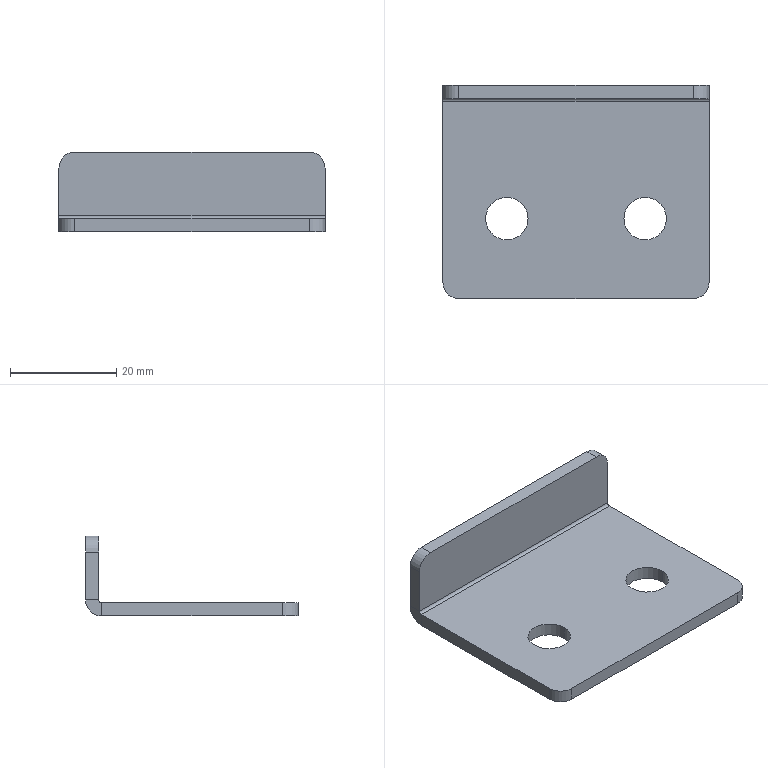Part | SolidWorks | features BaseBody 1 | 1 solid | 22 faces | box 50 x 40 x 15 mm | volume 6198 mm3 | plane 12 | cylinder 10 | commonest cylinder face diameters 6 x5 8 x4 1 x1
STEP:
#1=CARTESIAN_POINT('',(-17.,-5.,-2.5));
#2=VERTEX_POINT('',#1);
#3=CARTESIAN_POINT('',(-17.,-5.,0.));
#4=VERTEX_POINT('',#3);
#5=CARTESIAN_POINT('',(-17.,-5.,-2.5));
#6=DIRECTION('',(0.,0.,1.));
#7=VECTOR('',#6,1000.);
#8=LINE('',#5,#7);
#9=EDGE_CURVE('',#2,#4,#8,.T.);
#10=ORIENTED_EDGE('',*,*,#9,.F.);
#11=CARTESIAN_POINT('',(-9.,-5.,-2.5));
#12=VERTEX_POINT('',#11);
#13=CARTESIAN_POINT('',(-13.,-5.,-2.5));
#14=DIRECTION('',(0.,0.,1.));
#15=DIRECTION('',(1.,0.,0.));
#16=AXIS2_PLACEMENT_3D('',#13,#14,#15);
#17=CIRCLE('',#16,4.);
#18=EDGE_CURVE('',#12,#2,#17,.T.);
#19=ORIENTED_EDGE('',*,*,#18,.F.);
#20=CARTESIAN_POINT('',(-9.,-5.,0.));
#21=VERTEX_POINT('',#20);
#22=CARTESIAN_POINT('',(-9.,-5.,-2.5));
#23=DIRECTION('',(0.,0.,1.));
#24=VECTOR('',#23,1000.);
#25=LINE('',#22,#24);
#26=EDGE_CURVE('',#12,#21,#25,.T.);
#27=ORIENTED_EDGE('',*,*,#26,.T.);
#28=CARTESIAN_POINT('',(-13.,-5.,0.));
#29=DIRECTION('',(0.,0.,1.));
#30=DIRECTION('',(1.,0.,0.));
#31=AXIS2_PLACEMENT_3D('',#28,#29,#30);
#32=CIRCLE('',#31,4.);
#33=EDGE_CURVE('',#21,#4,#32,.T.);
#34=ORIENTED_EDGE('',*,*,#33,.T.);
#35=EDGE_LOOP('',(#10,#19,#27,#34));
#36=FACE_OUTER_BOUND('',#35,.T.);
#37=CARTESIAN_POINT('',(-13.,-5.,-2.5));
#38=DIRECTION('',(0.,0.,1.));
#39=DIRECTION('',(1.,0.,0.));
#40=AXIS2_PLACEMENT_3D('',#37,#38,#39);
#41=CYLINDRICAL_SURFACE('',#40,4.);
#42=ADVANCED_FACE('',(#36),#41,.F.);
#43=CARTESIAN_POINT('',(9.,-5.,-2.5));
#44=VERTEX_POINT('',#43);
#45=CARTESIAN_POINT('',(9.,-5.,0.));
#46=VERTEX_POINT('',#45);
#47=CARTESIAN_POINT('',(9.,-5.,-2.5));
#48=DIRECTION('',(0.,0.,1.));
#49=VECTOR('',#48,1000.);
#50=LINE('',#47,#49);
#51=EDGE_CURVE('',#44,#46,#50,.T.);
#52=ORIENTED_EDGE('',*,*,#51,.F.);
#53=CARTESIAN_POINT('',(17.,-5.,-2.5));
#54=VERTEX_POINT('',#53);
#55=CARTESIAN_POINT('',(13.,-5.,-2.5));
#56=DIRECTION('',(0.,0.,1.));
#57=DIRECTION('',(1.,0.,0.));
#58=AXIS2_PLACEMENT_3D('',#55,#56,#57);
#59=CIRCLE('',#58,4.);
#60=EDGE_CURVE('',#54,#44,#59,.T.);
#61=ORIENTED_EDGE('',*,*,#60,.F.);
#62=CARTESIAN_POINT('',(17.,-5.,0.));
#63=VERTEX_POINT('',#62);
#64=CARTESIAN_POINT('',(17.,-5.,-2.5));
#65=DIRECTION('',(0.,0.,1.));
#66=VECTOR('',#65,1000.);
#67=LINE('',#64,#66);
#68=EDGE_CURVE('',#54,#63,#67,.T.);
#69=ORIENTED_EDGE('',*,*,#68,.T.);
#70=CARTESIAN_POINT('',(13.,-5.,0.));
#71=DIRECTION('',(0.,0.,1.));
#72=DIRECTION('',(1.,0.,0.));
#73=AXIS2_PLACEMENT_3D('',#70,#71,#72);
#74=CIRCLE('',#73,4.);
#75=EDGE_CURVE('',#63,#46,#74,.T.);
#76=ORIENTED_EDGE('',*,*,#75,.T.);
#77=EDGE_LOOP('',(#52,#61,#69,#76));
#78=FACE_OUTER_BOUND('',#77,.T.);
#79=CARTESIAN_POINT('',(13.,-5.,-2.5));
#80=DIRECTION('',(0.,0.,1.));
#81=DIRECTION('',(1.,0.,0.));
#82=AXIS2_PLACEMENT_3D('',#79,#80,#81);
#83=CYLINDRICAL_SURFACE('',#82,4.);
#84=ADVANCED_FACE('',(#78),#83,.F.);
#85=CARTESIAN_POINT('',(-25.,20.,9.5));
#86=VERTEX_POINT('',#85);
#87=CARTESIAN_POINT('',(-22.,20.,12.5));
#88=VERTEX_POINT('',#87);
#89=CARTESIAN_POINT('',(-22.,20.,9.5));
#90=DIRECTION('',(0.,1.,0.));
#91=DIRECTION('',(0.,0.,-1.));
#92=AXIS2_PLACEMENT_3D('',#89,#90,#91);
#93=CIRCLE('',#92,3.);
#94=EDGE_CURVE('',#86,#88,#93,.T.);
#95=ORIENTED_EDGE('',*,*,#94,.F.);
#96=CARTESIAN_POINT('',(-25.,17.5,9.5));
#97=VERTEX_POINT('',#96);
#98=CARTESIAN_POINT('',(-25.,20.,9.5));
#99=DIRECTION('',(0.,1.,0.));
#100=VECTOR('',#99,1000.);
#101=LINE('',#98,#100);
#102=EDGE_CURVE('',#97,#86,#101,.T.);
#103=ORIENTED_EDGE('',*,*,#102,.F.);
#104=CARTESIAN_POINT('',(-22.,17.5,12.5));
#105=VERTEX_POINT('',#104);
#106=CARTESIAN_POINT('',(-22.,17.5,9.5));
#107=DIRECTION('',(0.,-1.,0.));
#108=DIRECTION('',(0.,0.,-1.));
#109=AXIS2_PLACEMENT_3D('',#106,#107,#108);
#110=CIRCLE('',#109,3.);
#111=EDGE_CURVE('',#105,#97,#110,.T.);
#112=ORIENTED_EDGE('',*,*,#111,.F.);
#113=CARTESIAN_POINT('',(-22.,20.,12.5));
#114=DIRECTION('',(0.,-1.,0.));
#115=VECTOR('',#114,1000.);
#116=LINE('',#113,#115);
#117=EDGE_CURVE('',#88,#105,#116,.T.);
#118=ORIENTED_EDGE('',*,*,#117,.F.);
#119=EDGE_LOOP('',(#95,#103,#112,#118));
#120=FACE_OUTER_BOUND('',#119,.T.);
#121=CARTESIAN_POINT('',(-22.,20.,9.5));
#122=DIRECTION('',(0.,-1.,0.));
#123=DIRECTION('',(0.,0.,-1.));
#124=AXIS2_PLACEMENT_3D('',#121,#122,#123);
#125=CYLINDRICAL_SURFACE('',#124,3.);
#126=ADVANCED_FACE('',(#120),#125,.T.);
#127=CARTESIAN_POINT('',(22.,20.,12.5));
#128=VERTEX_POINT('',#127);
#129=CARTESIAN_POINT('',(25.,20.,9.5));
#130=VERTEX_POINT('',#129);
#131=CARTESIAN_POINT('',(22.,20.,9.5));
#132=DIRECTION('',(0.,1.,0.));
#133=DIRECTION('',(0.,0.,-1.));
#134=AXIS2_PLACEMENT_3D('',#131,#132,#133);
#135=CIRCLE('',#134,3.);
#136=EDGE_CURVE('',#128,#130,#135,.T.);
#137=ORIENTED_EDGE('',*,*,#136,.F.);
#138=CARTESIAN_POINT('',(22.,17.5,12.5));
#139=VERTEX_POINT('',#138);
#140=CARTESIAN_POINT('',(22.,20.,12.5));
#141=DIRECTION('',(0.,1.,0.));
#142=VECTOR('',#141,1000.);
#143=LINE('',#140,#142);
#144=EDGE_CURVE('',#139,#128,#143,.T.);
#145=ORIENTED_EDGE('',*,*,#144,.F.);
#146=CARTESIAN_POINT('',(25.,17.5,9.5));
#147=VERTEX_POINT('',#146);
#148=CARTESIAN_POINT('',(22.,17.5,9.5));
#149=DIRECTION('',(0.,-1.,0.));
#150=DIRECTION('',(0.,0.,-1.));
#151=AXIS2_PLACEMENT_3D('',#148,#149,#150);
#152=CIRCLE('',#151,3.);
#153=EDGE_CURVE('',#147,#139,#152,.T.);
#154=ORIENTED_EDGE('',*,*,#153,.F.);
#155=CARTESIAN_POINT('',(25.,20.,9.5));
#156=DIRECTION('',(0.,-1.,0.));
#157=VECTOR('',#156,1000.);
#158=LINE('',#155,#157);
#159=EDGE_CURVE('',#130,#147,#158,.T.);
#160=ORIENTED_EDGE('',*,*,#159,.F.);
#161=EDGE_LOOP('',(#137,#145,#154,#160));
#162=FACE_OUTER_BOUND('',#161,.T.);
#163=CARTESIAN_POINT('',(22.,20.,9.5));
#164=DIRECTION('',(0.,-1.,0.));
#165=DIRECTION('',(0.,0.,-1.));
#166=AXIS2_PLACEMENT_3D('',#163,#164,#165);
#167=CYLINDRICAL_SURFACE('',#166,3.);
#168=ADVANCED_FACE('',(#162),#167,.T.);
#169=CARTESIAN_POINT('',(-22.,-20.,-2.5));
#170=VERTEX_POINT('',#169);
#171=CARTESIAN_POINT('',(-25.,-17.,-2.5));
#172=VERTEX_POINT('',#171);
#173=CARTESIAN_POINT('',(-22.,-17.,-2.5));
#174=DIRECTION('',(0.,0.,-1.));
#175=DIRECTION('',(-1.,0.,0.));
#176=AXIS2_PLACEMENT_3D('',#173,#174,#175);
#177=CIRCLE('',#176,3.);
#178=EDGE_CURVE('',#170,#172,#177,.T.);
#179=ORIENTED_EDGE('',*,*,#178,.F.);
#180=CARTESIAN_POINT('',(-22.,-20.,0.));
#181=VERTEX_POINT('',#180);
#182=CARTESIAN_POINT('',(-22.,-20.,-2.5));
#183=DIRECTION('',(0.,0.,-1.));
#184=VECTOR('',#183,1000.);
#185=LINE('',#182,#184);
#186=EDGE_CURVE('',#181,#170,#185,.T.);
#187=ORIENTED_EDGE('',*,*,#186,.F.);
#188=CARTESIAN_POINT('',(-25.,-17.,0.));
#189=VERTEX_POINT('',#188);
#190=CARTESIAN_POINT('',(-22.,-17.,0.));
#191=DIRECTION('',(0.,0.,1.));
#192=DIRECTION('',(-1.,0.,0.));
#193=AXIS2_PLACEMENT_3D('',#190,#191,#192);
#194=CIRCLE('',#193,3.);
#195=EDGE_CURVE('',#189,#181,#194,.T.);
#196=ORIENTED_EDGE('',*,*,#195,.F.);
#197=CARTESIAN_POINT('',(-25.,-17.,-2.5));
#198=DIRECTION('',(0.,0.,1.));
#199=VECTOR('',#198,1000.);
#200=LINE('',#197,#199);
#201=EDGE_CURVE('',#172,#189,#200,.T.);
#202=ORIENTED_EDGE('',*,*,#201,.F.);
#203=EDGE_LOOP('',(#179,#187,#196,#202));
#204=FACE_OUTER_BOUND('',#203,.T.);
#205=CARTESIAN_POINT('',(-22.,-17.,-2.5));
#206=DIRECTION('',(0.,0.,1.));
#207=DIRECTION('',(1.,0.,0.));
#208=AXIS2_PLACEMENT_3D('',#205,#206,#207);
#209=CYLINDRICAL_SURFACE('',#208,3.);
#210=ADVANCED_FACE('',(#204),#209,.T.);
#211=CARTESIAN_POINT('',(25.,-17.,-2.5));
#212=VERTEX_POINT('',#211);
#213=CARTESIAN_POINT('',(22.,-20.,-2.5));
#214=VERTEX_POINT('',#213);
#215=CARTESIAN_POINT('',(22.,-17.,-2.5));
#216=DIRECTION('',(0.,0.,-1.));
#217=DIRECTION('',(-1.,0.,0.));
#218=AXIS2_PLACEMENT_3D('',#215,#216,#217);
#219=CIRCLE('',#218,3.);
#220=EDGE_CURVE('',#212,#214,#219,.T.);
#221=ORIENTED_EDGE('',*,*,#220,.F.);
#222=CARTESIAN_POINT('',(25.,-17.,0.));
#223=VERTEX_POINT('',#222);
#224=CARTESIAN_POINT('',(25.,-17.,-2.5));
#225=DIRECTION('',(0.,0.,-1.));
#226=VECTOR('',#225,1000.);
#227=LINE('',#224,#226);
#228=EDGE_CURVE('',#223,#212,#227,.T.);
#229=ORIENTED_EDGE('',*,*,#228,.F.);
#230=CARTESIAN_POINT('',(22.,-20.,0.));
#231=VERTEX_POINT('',#230);
#232=CARTESIAN_POINT('',(22.,-17.,0.));
#233=DIRECTION('',(0.,0.,1.));
#234=DIRECTION('',(-1.,0.,0.));
#235=AXIS2_PLACEMENT_3D('',#232,#233,#234);
#236=CIRCLE('',#235,3.);
#237=EDGE_CURVE('',#231,#223,#236,.T.);
#238=ORIENTED_EDGE('',*,*,#237,.F.);
#239=CARTESIAN_POINT('',(22.,-20.,-2.5));
#240=DIRECTION('',(0.,0.,1.));
#241=VECTOR('',#240,1000.);
#242=LINE('',#239,#241);
#243=EDGE_CURVE('',#214,#231,#242,.T.);
#244=ORIENTED_EDGE('',*,*,#243,.F.);
#245=EDGE_LOOP('',(#221,#229,#238,#244));
#246=FACE_OUTER_BOUND('',#245,.T.);
#247=CARTESIAN_POINT('',(22.,-17.,-2.5));
#248=DIRECTION('',(0.,0.,1.));
#249=DIRECTION('',(1.,0.,0.));
#250=AXIS2_PLACEMENT_3D('',#247,#248,#249);
#251=CYLINDRICAL_SURFACE('',#250,3.);
#252=ADVANCED_FACE('',(#246),#251,.T.);
#253=CARTESIAN_POINT('',(25.,17.5,12.5));
#254=DIRECTION('',(1.,0.,0.));
#255=VECTOR('',#254,1000.);
#256=LINE('',#253,#255);
#257=EDGE_CURVE('',#105,#139,#256,.T.);
#258=ORIENTED_EDGE('',*,*,#257,.T.);
#259=ORIENTED_EDGE('',*,*,#144,.T.);
#260=CARTESIAN_POINT('',(0.,20.,12.5));
#261=DIRECTION('',(1.,0.,0.));
#262=VECTOR('',#261,1000.);
#263=LINE('',#260,#262);
#264=EDGE_CURVE('',#88,#128,#263,.T.);
#265=ORIENTED_EDGE('',*,*,#264,.F.);
#266=ORIENTED_EDGE('',*,*,#117,.T.);
#267=EDGE_LOOP('',(#258,#259,#265,#266));
#268=FACE_OUTER_BOUND('',#267,.T.);
#269=CARTESIAN_POINT('',(25.,20.,12.5));
#270=DIRECTION('',(0.,0.,-1.));
#271=DIRECTION('',(0.,-1.,0.));
#272=AXIS2_PLACEMENT_3D('',#269,#270,#271);
#273=PLANE('',#272);
#274=ADVANCED_FACE('',(#268),#273,.F.);
#275=CARTESIAN_POINT('',(25.,17.5,0.5));
#276=VERTEX_POINT('',#275);
#277=CARTESIAN_POINT('',(25.,17.5,0.));
#278=DIRECTION('',(0.,0.,-1.));
#279=VECTOR('',#278,1000.);
#280=LINE('',#277,#279);
#281=EDGE_CURVE('',#147,#276,#280,.T.);
#282=ORIENTED_EDGE('',*,*,#281,.F.);
#283=ORIENTED_EDGE('',*,*,#153,.T.);
#284=ORIENTED_EDGE('',*,*,#257,.F.);
#285=ORIENTED_EDGE('',*,*,#111,.T.);
#286=CARTESIAN_POINT('',(-25.,17.5,0.5));
#287=VERTEX_POINT('',#286);
#288=CARTESIAN_POINT('',(-25.,17.5,12.5));
#289=DIRECTION('',(0.,0.,1.));
#290=VECTOR('',#289,1000.);
#291=LINE('',#288,#290);
#292=EDGE_CURVE('',#287,#97,#291,.T.);
#293=ORIENTED_EDGE('',*,*,#292,.F.);
#294=CARTESIAN_POINT('',(25.,17.5,0.5));
#295=DIRECTION('',(-1.,0.,0.));
#296=VECTOR('',#295,1000.);
#297=LINE('',#294,#296);
#298=EDGE_CURVE('',#276,#287,#297,.T.);
#299=ORIENTED_EDGE('',*,*,#298,.F.);
#300=EDGE_LOOP('',(#282,#283,#284,#285,#293,#299));
#301=FACE_OUTER_BOUND('',#300,.T.);
#302=CARTESIAN_POINT('',(0.,17.5,0.));
#303=DIRECTION('',(0.,-1.,0.));
#304=DIRECTION('',(-1.,0.,0.));
#305=AXIS2_PLACEMENT_3D('',#302,#303,#304);
#306=PLANE('',#305);
#307=ADVANCED_FACE('',(#301),#306,.T.);
#308=ORIENTED_EDGE('',*,*,#264,.T.);
#309=ORIENTED_EDGE('',*,*,#136,.T.);
#310=CARTESIAN_POINT('',(25.,20.,0.5));
#311=VERTEX_POINT('',#310);
#312=CARTESIAN_POINT('',(25.,20.,0.));
#313=DIRECTION('',(0.,0.,-1.));
#314=VECTOR('',#313,1000.);
#315=LINE('',#312,#314);
#316=EDGE_CURVE('',#130,#311,#315,.T.);
#317=ORIENTED_EDGE('',*,*,#316,.T.);
#318=CARTESIAN_POINT('',(-25.,20.,0.5));
#319=VERTEX_POINT('',#318);
#320=CARTESIAN_POINT('',(25.,20.,0.5));
#321=DIRECTION('',(1.,0.,0.));
#322=VECTOR('',#321,1000.);
#323=LINE('',#320,#322);
#324=EDGE_CURVE('',#319,#311,#323,.T.);
#325=ORIENTED_EDGE('',*,*,#324,.F.);
#326=CARTESIAN_POINT('',(-25.,20.,0.));
#327=DIRECTION('',(0.,0.,1.));
#328=VECTOR('',#327,1000.);
#329=LINE('',#326,#328);
#330=EDGE_CURVE('',#319,#86,#329,.T.);
#331=ORIENTED_EDGE('',*,*,#330,.T.);
#332=ORIENTED_EDGE('',*,*,#94,.T.);
#333=EDGE_LOOP('',(#308,#309,#317,#325,#331,#332));
#334=FACE_OUTER_BOUND('',#333,.T.);
#335=CARTESIAN_POINT('',(0.,20.,0.));
#336=DIRECTION('',(0.,-1.,0.));
#337=DIRECTION('',(-1.,0.,0.));
#338=AXIS2_PLACEMENT_3D('',#335,#336,#337);
#339=PLANE('',#338);
#340=ADVANCED_FACE('',(#334),#339,.F.);
#341=ORIENTED_EDGE('',*,*,#292,.T.);
#342=ORIENTED_EDGE('',*,*,#102,.T.);
#343=ORIENTED_EDGE('',*,*,#330,.F.);
#344=CARTESIAN_POINT('',(-25.,17.5,0.5));
#345=DIRECTION('',(0.,1.,0.));
#346=VECTOR('',#345,1000.);
#347=LINE('',#344,#346);
#348=EDGE_CURVE('',#287,#319,#347,.T.);
#349=ORIENTED_EDGE('',*,*,#348,.F.);
#350=EDGE_LOOP('',(#341,#342,#343,#349));
#351=FACE_OUTER_BOUND('',#350,.T.);
#352=CARTESIAN_POINT('',(-25.,20.,12.5));
#353=DIRECTION('',(1.,0.,0.));
#354=DIRECTION('',(0.,1.,0.));
#355=AXIS2_PLACEMENT_3D('',#352,#353,#354);
#356=PLANE('',#355);
#357=ADVANCED_FACE('',(#351),#356,.F.);
#358=ORIENTED_EDGE('',*,*,#316,.F.);
#359=ORIENTED_EDGE('',*,*,#159,.T.);
#360=ORIENTED_EDGE('',*,*,#281,.T.);
#361=CARTESIAN_POINT('',(25.,20.,0.5));
#362=DIRECTION('',(0.,1.,0.));
#363=VECTOR('',#362,1000.);
#364=LINE('',#361,#363);
#365=EDGE_CURVE('',#276,#311,#364,.T.);
#366=ORIENTED_EDGE('',*,*,#365,.T.);
#367=EDGE_LOOP('',(#358,#359,#360,#366));
#368=FACE_OUTER_BOUND('',#367,.T.);
#369=CARTESIAN_POINT('',(25.,20.,0.));
#370=DIRECTION('',(-1.,0.,0.));
#371=DIRECTION('',(0.,1.,0.));
#372=AXIS2_PLACEMENT_3D('',#369,#370,#371);
#373=PLANE('',#372);
#374=ADVANCED_FACE('',(#368),#373,.F.);
#375=CARTESIAN_POINT('',(-25.,17.,0.));
#376=VERTEX_POINT('',#375);
#377=CARTESIAN_POINT('',(25.,17.,0.));
#378=VERTEX_POINT('',#377);
#379=CARTESIAN_POINT('',(-25.,17.,0.));
#380=DIRECTION('',(1.,0.,0.));
#381=VECTOR('',#380,1000.);
#382=LINE('',#379,#381);
#383=EDGE_CURVE('',#376,#378,#382,.T.);
#384=ORIENTED_EDGE('',*,*,#383,.T.);
#385=CARTESIAN_POINT('',(25.,17.,0.5));
#386=DIRECTION('',(1.,0.,0.));
#387=DIRECTION('',(0.,0.,1.));
#388=AXIS2_PLACEMENT_3D('',#385,#386,#387);
#389=CIRCLE('',#388,0.5);
#390=EDGE_CURVE('',#378,#276,#389,.T.);
#391=ORIENTED_EDGE('',*,*,#390,.T.);
#392=ORIENTED_EDGE('',*,*,#298,.T.);
#393=CARTESIAN_POINT('',(-25.,17.,0.5));
#394=DIRECTION('',(-1.,0.,0.));
#395=DIRECTION('',(0.,0.,1.));
#396=AXIS2_PLACEMENT_3D('',#393,#394,#395);
#397=CIRCLE('',#396,0.5);
#398=EDGE_CURVE('',#287,#376,#397,.T.);
#399=ORIENTED_EDGE('',*,*,#398,.T.);
#400=EDGE_LOOP('',(#384,#391,#392,#399));
#401=FACE_OUTER_BOUND('',#400,.T.);
#402=CARTESIAN_POINT('',(-25.,17.,0.5));
#403=DIRECTION('',(-1.,0.,0.));
#404=DIRECTION('',(0.,1.,0.));
#405=AXIS2_PLACEMENT_3D('',#402,#403,#404);
#406=CYLINDRICAL_SURFACE('',#405,0.5);
#407=ADVANCED_FACE('',(#401),#406,.F.);
#408=CARTESIAN_POINT('',(-25.,17.,-2.5));
#409=VERTEX_POINT('',#408);
#410=CARTESIAN_POINT('',(25.,17.,-2.5));
#411=VERTEX_POINT('',#410);
#412=CARTESIAN_POINT('',(-25.,17.,-2.5));
#413=DIRECTION('',(1.,0.,0.));
#414=VECTOR('',#413,1000.);
#415=LINE('',#412,#414);
#416=EDGE_CURVE('',#409,#411,#415,.T.);
#417=ORIENTED_EDGE('',*,*,#416,.F.);
#418=CARTESIAN_POINT('',(-25.,17.,0.5));
#419=DIRECTION('',(-1.,0.,0.));
#420=DIRECTION('',(0.,0.,1.));
#421=AXIS2_PLACEMENT_3D('',#418,#419,#420);
#422=CIRCLE('',#421,3.);
#423=EDGE_CURVE('',#319,#409,#422,.T.);
#424=ORIENTED_EDGE('',*,*,#423,.F.);
#425=ORIENTED_EDGE('',*,*,#324,.T.);
#426=CARTESIAN_POINT('',(25.,17.,0.5));
#427=DIRECTION('',(1.,0.,0.));
#428=DIRECTION('',(0.,0.,1.));
#429=AXIS2_PLACEMENT_3D('',#426,#427,#428);
#430=CIRCLE('',#429,3.);
#431=EDGE_CURVE('',#411,#311,#430,.T.);
#432=ORIENTED_EDGE('',*,*,#431,.F.);
#433=EDGE_LOOP('',(#417,#424,#425,#432));
#434=FACE_OUTER_BOUND('',#433,.T.);
#435=CARTESIAN_POINT('',(-25.,17.,0.5));
#436=DIRECTION('',(-1.,0.,0.));
#437=DIRECTION('',(0.,1.,0.));
#438=AXIS2_PLACEMENT_3D('',#435,#436,#437);
#439=CYLINDRICAL_SURFACE('',#438,3.);
#440=ADVANCED_FACE('',(#434),#439,.T.);
#441=ORIENTED_EDGE('',*,*,#398,.F.);
#442=ORIENTED_EDGE('',*,*,#348,.T.);
#443=ORIENTED_EDGE('',*,*,#423,.T.);
#444=CARTESIAN_POINT('',(-25.,17.,0.));
#445=DIRECTION('',(0.,0.,-1.));
#446=VECTOR('',#445,1000.);
#447=LINE('',#444,#446);
#448=EDGE_CURVE('',#376,#409,#447,.T.);
#449=ORIENTED_EDGE('',*,*,#448,.F.);
#450=EDGE_LOOP('',(#441,#442,#443,#449));
#451=FACE_OUTER_BOUND('',#450,.T.);
#452=CARTESIAN_POINT('',(-25.,17.,0.5));
#453=DIRECTION('',(1.,0.,0.));
#454=DIRECTION('',(0.,1.,0.));
#455=AXIS2_PLACEMENT_3D('',#452,#453,#454);
#456=PLANE('',#455);
#457=ADVANCED_FACE('',(#451),#456,.F.);
#458=ORIENTED_EDGE('',*,*,#365,.F.);
#459=ORIENTED_EDGE('',*,*,#390,.F.);
#460=CARTESIAN_POINT('',(25.,17.,0.));
#461=DIRECTION('',(0.,0.,-1.));
#462=VECTOR('',#461,1000.);
#463=LINE('',#460,#462);
#464=EDGE_CURVE('',#378,#411,#463,.T.);
#465=ORIENTED_EDGE('',*,*,#464,.T.);
#466=ORIENTED_EDGE('',*,*,#431,.T.);
#467=EDGE_LOOP('',(#458,#459,#465,#466));
#468=FACE_OUTER_BOUND('',#467,.T.);
#469=CARTESIAN_POINT('',(25.,17.,0.5));
#470=DIRECTION('',(1.,0.,0.));
#471=DIRECTION('',(0.,1.,0.));
#472=AXIS2_PLACEMENT_3D('',#469,#470,#471);
#473=PLANE('',#472);
#474=ADVANCED_FACE('',(#468),#473,.T.);
#475=CARTESIAN_POINT('',(25.,-20.,-2.5));
#476=DIRECTION('',(1.,0.,0.));
#477=VECTOR('',#476,1000.);
#478=LINE('',#475,#477);
#479=EDGE_CURVE('',#170,#214,#478,.T.);
#480=ORIENTED_EDGE('',*,*,#479,.T.);
#481=ORIENTED_EDGE('',*,*,#243,.T.);
#482=CARTESIAN_POINT('',(25.,-20.,0.));
#483=DIRECTION('',(1.,0.,0.));
#484=VECTOR('',#483,1000.);
#485=LINE('',#482,#484);
#486=EDGE_CURVE('',#181,#231,#485,.T.);
#487=ORIENTED_EDGE('',*,*,#486,.F.);
#488=ORIENTED_EDGE('',*,*,#186,.T.);
#489=EDGE_LOOP('',(#480,#481,#487,#488));
#490=FACE_OUTER_BOUND('',#489,.T.);
#491=CARTESIAN_POINT('',(25.,-20.,-2.5));
#492=DIRECTION('',(0.,-1.,0.));
#493=DIRECTION('',(0.,0.,-1.));
#494=AXIS2_PLACEMENT_3D('',#491,#492,#493);
#495=PLANE('',#494);
#496=ADVANCED_FACE('',(#490),#495,.T.);
#497=CARTESIAN_POINT('',(25.,20.,0.));
#498=DIRECTION('',(0.,1.,0.));
#499=VECTOR('',#498,1000.);
#500=LINE('',#497,#499);
#501=EDGE_CURVE('',#223,#378,#500,.T.);
#502=ORIENTED_EDGE('',*,*,#501,.F.);
#503=ORIENTED_EDGE('',*,*,#228,.T.);
#504=CARTESIAN_POINT('',(25.,20.,-2.5));
#505=DIRECTION('',(0.,1.,0.));
#506=VECTOR('',#505,1000.);
#507=LINE('',#504,#506);
#508=EDGE_CURVE('',#212,#411,#507,.T.);
#509=ORIENTED_EDGE('',*,*,#508,.T.);
#510=ORIENTED_EDGE('',*,*,#464,.F.);
#511=EDGE_LOOP('',(#502,#503,#509,#510));
#512=FACE_OUTER_BOUND('',#511,.T.);
#513=CARTESIAN_POINT('',(25.,20.,-2.5));
#514=DIRECTION('',(1.,0.,0.));
#515=DIRECTION('',(0.,1.,0.));
#516=AXIS2_PLACEMENT_3D('',#513,#514,#515);
#517=PLANE('',#516);
#518=ADVANCED_FACE('',(#512),#517,.T.);
#519=ORIENTED_EDGE('',*,*,#75,.F.);
#520=CARTESIAN_POINT('',(13.,-5.,0.));
#521=DIRECTION('',(0.,0.,1.));
#522=DIRECTION('',(1.,0.,0.));
#523=AXIS2_PLACEMENT_3D('',#520,#521,#522);
#524=CIRCLE('',#523,4.);
#525=EDGE_CURVE('',#46,#63,#524,.T.);
#526=ORIENTED_EDGE('',*,*,#525,.F.);
#527=EDGE_LOOP('',(#519,#526));
#528=FACE_BOUND('',#527,.T.);
#529=ORIENTED_EDGE('',*,*,#33,.F.);
#530=CARTESIAN_POINT('',(-13.,-5.,0.));
#531=DIRECTION('',(0.,0.,1.));
#532=DIRECTION('',(1.,0.,0.));
#533=AXIS2_PLACEMENT_3D('',#530,#531,#532);
#534=CIRCLE('',#533,4.);
#535=EDGE_CURVE('',#4,#21,#534,.T.);
#536=ORIENTED_EDGE('',*,*,#535,.F.);
#537=EDGE_LOOP('',(#529,#536));
#538=FACE_BOUND('',#537,.T.);
#539=ORIENTED_EDGE('',*,*,#486,.T.);
#540=ORIENTED_EDGE('',*,*,#237,.T.);
#541=ORIENTED_EDGE('',*,*,#501,.T.);
#542=ORIENTED_EDGE('',*,*,#383,.F.);
#543=CARTESIAN_POINT('',(-25.,20.,0.));
#544=DIRECTION('',(0.,-1.,0.));
#545=VECTOR('',#544,1000.);
#546=LINE('',#543,#545);
#547=EDGE_CURVE('',#376,#189,#546,.T.);
#548=ORIENTED_EDGE('',*,*,#547,.T.);
#549=ORIENTED_EDGE('',*,*,#195,.T.);
#550=EDGE_LOOP('',(#539,#540,#541,#542,#548,#549));
#551=FACE_OUTER_BOUND('',#550,.T.);
#552=CARTESIAN_POINT('',(0.,0.,0.));
#553=DIRECTION('',(0.,0.,-1.));
#554=DIRECTION('',(0.,-1.,0.));
#555=AXIS2_PLACEMENT_3D('',#552,#553,#554);
#556=PLANE('',#555);
#557=ADVANCED_FACE('',(#528,#538,#551),#556,.F.);
#558=ORIENTED_EDGE('',*,*,#60,.T.);
#559=CARTESIAN_POINT('',(13.,-5.,-2.5));
#560=DIRECTION('',(0.,0.,1.));
#561=DIRECTION('',(1.,0.,0.));
#562=AXIS2_PLACEMENT_3D('',#559,#560,#561);
#563=CIRCLE('',#562,4.);
#564=EDGE_CURVE('',#44,#54,#563,.T.);
#565=ORIENTED_EDGE('',*,*,#564,.T.);
#566=EDGE_LOOP('',(#558,#565));
#567=FACE_BOUND('',#566,.T.);
#568=ORIENTED_EDGE('',*,*,#18,.T.);
#569=CARTESIAN_POINT('',(-13.,-5.,-2.5));
#570=DIRECTION('',(0.,0.,1.));
#571=DIRECTION('',(1.,0.,0.));
#572=AXIS2_PLACEMENT_3D('',#569,#570,#571);
#573=CIRCLE('',#572,4.);
#574=EDGE_CURVE('',#2,#12,#573,.T.);
#575=ORIENTED_EDGE('',*,*,#574,.T.);
#576=EDGE_LOOP('',(#568,#575));
#577=FACE_BOUND('',#576,.T.);
#578=ORIENTED_EDGE('',*,*,#508,.F.);
#579=ORIENTED_EDGE('',*,*,#220,.T.);
#580=ORIENTED_EDGE('',*,*,#479,.F.);
#581=ORIENTED_EDGE('',*,*,#178,.T.);
#582=CARTESIAN_POINT('',(-25.,20.,-2.5));
#583=DIRECTION('',(0.,-1.,0.));
#584=VECTOR('',#583,1000.);
#585=LINE('',#582,#584);
#586=EDGE_CURVE('',#409,#172,#585,.T.);
#587=ORIENTED_EDGE('',*,*,#586,.F.);
#588=ORIENTED_EDGE('',*,*,#416,.T.);
#589=EDGE_LOOP('',(#578,#579,#580,#581,#587,#588));
#590=FACE_OUTER_BOUND('',#589,.T.);
#591=CARTESIAN_POINT('',(0.,0.,-2.5));
#592=DIRECTION('',(0.,0.,-1.));
#593=DIRECTION('',(0.,-1.,0.));
#594=AXIS2_PLACEMENT_3D('',#591,#592,#593);
#595=PLANE('',#594);
#596=ADVANCED_FACE('',(#567,#577,#590),#595,.T.);
#597=ORIENTED_EDGE('',*,*,#586,.T.);
#598=ORIENTED_EDGE('',*,*,#201,.T.);
#599=ORIENTED_EDGE('',*,*,#547,.F.);
#600=ORIENTED_EDGE('',*,*,#448,.T.);
#601=EDGE_LOOP('',(#597,#598,#599,#600));
#602=FACE_OUTER_BOUND('',#601,.T.);
#603=CARTESIAN_POINT('',(-25.,20.,-2.5));
#604=DIRECTION('',(-1.,0.,0.));
#605=DIRECTION('',(0.,1.,0.));
#606=AXIS2_PLACEMENT_3D('',#603,#604,#605);
#607=PLANE('',#606);
#608=ADVANCED_FACE('',(#602),#607,.T.);
#609=ORIENTED_EDGE('',*,*,#564,.F.);
#610=ORIENTED_EDGE('',*,*,#51,.T.);
#611=ORIENTED_EDGE('',*,*,#525,.T.);
#612=ORIENTED_EDGE('',*,*,#68,.F.);
#613=EDGE_LOOP('',(#609,#610,#611,#612));
#614=FACE_OUTER_BOUND('',#613,.T.);
#615=CARTESIAN_POINT('',(13.,-5.,-2.5));
#616=DIRECTION('',(0.,0.,1.));
#617=DIRECTION('',(1.,0.,0.));
#618=AXIS2_PLACEMENT_3D('',#615,#616,#617);
#619=CYLINDRICAL_SURFACE('',#618,4.);
#620=ADVANCED_FACE('',(#614),#619,.F.);
#621=ORIENTED_EDGE('',*,*,#574,.F.);
#622=ORIENTED_EDGE('',*,*,#9,.T.);
#623=ORIENTED_EDGE('',*,*,#535,.T.);
#624=ORIENTED_EDGE('',*,*,#26,.F.);
#625=EDGE_LOOP('',(#621,#622,#623,#624));
#626=FACE_OUTER_BOUND('',#625,.T.);
#627=CARTESIAN_POINT('',(-13.,-5.,-2.5));
#628=DIRECTION('',(0.,0.,1.));
#629=DIRECTION('',(1.,0.,0.));
#630=AXIS2_PLACEMENT_3D('',#627,#628,#629);
#631=CYLINDRICAL_SURFACE('',#630,4.);
#632=ADVANCED_FACE('',(#626),#631,.F.);
#633=CLOSED_SHELL('',(#42,#84,#126,#168,#210,#252,#274,#307,#340,#357,#374,#407,#440,#457,#474,#496,#518,#557,#596,#608,#620,#632));
#634=MANIFOLD_SOLID_BREP('',#633);
#635=CARTESIAN_POINT('',(0.,0.,0.));
#636=DIRECTION('',(0.,0.,1.));
#637=DIRECTION('',(1.,0.,0.));
#638=AXIS2_PLACEMENT_3D('',#635,#636,#637);
#639=(LENGTH_UNIT()NAMED_UNIT(*)SI_UNIT(.MILLI.,.METRE.));
#640=UNCERTAINTY_MEASURE_WITH_UNIT(LENGTH_MEASURE(0.00001),#639,'','');
#641=(NAMED_UNIT(*)PLANE_ANGLE_UNIT()SI_UNIT($,.RADIAN.));
#642=(NAMED_UNIT(*)SI_UNIT($,.STERADIAN.)SOLID_ANGLE_UNIT());
#643=(GEOMETRIC_REPRESENTATION_CONTEXT(3)GLOBAL_UNCERTAINTY_ASSIGNED_CONTEXT((#640))GLOBAL_UNIT_ASSIGNED_CONTEXT((#639,#641,#642))REPRESENTATION_CONTEXT('',''));
#644=ADVANCED_BREP_SHAPE_REPRESENTATION('',(#634,#638),#643);